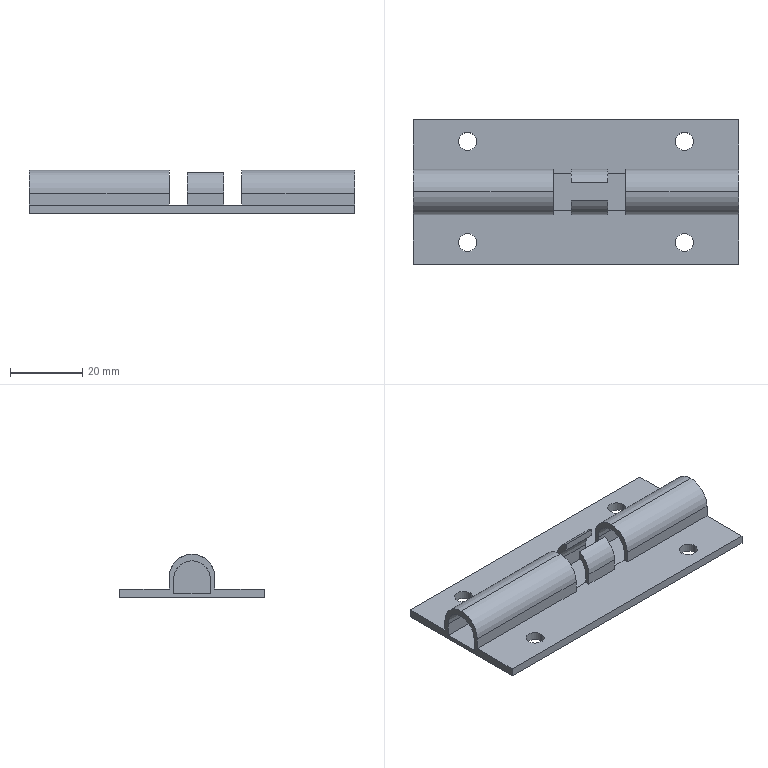Part | SolidWorks | features BaseBody 1 | 1 solid | 45 faces | box 90 x 40 x 12 mm | volume 11713 mm3 | plane 25 | cylinder 20 | commonest cylinder face diameters 5 x8 10.2 x6 12.6 x6
STEP:
#1=CARTESIAN_POINT('',(17.5,14.,2.4));
#2=VERTEX_POINT('',#1);
#3=CARTESIAN_POINT('',(12.5,14.,2.4));
#4=VERTEX_POINT('',#3);
#5=CARTESIAN_POINT('',(15.,14.,2.4));
#6=DIRECTION('',(0.,0.,-1.));
#7=DIRECTION('',(-1.,0.,0.));
#8=AXIS2_PLACEMENT_3D('',#5,#6,#7);
#9=CIRCLE('',#8,2.5);
#10=EDGE_CURVE('',#2,#4,#9,.T.);
#11=ORIENTED_EDGE('',*,*,#10,.F.);
#12=CARTESIAN_POINT('',(17.5,14.,0.));
#13=VERTEX_POINT('',#12);
#14=CARTESIAN_POINT('',(17.5,14.,0.));
#15=DIRECTION('',(0.,0.,-1.));
#16=VECTOR('',#15,1000.);
#17=LINE('',#14,#16);
#18=EDGE_CURVE('',#2,#13,#17,.T.);
#19=ORIENTED_EDGE('',*,*,#18,.T.);
#20=CARTESIAN_POINT('',(12.5,14.,0.));
#21=VERTEX_POINT('',#20);
#22=CARTESIAN_POINT('',(15.,14.,0.));
#23=DIRECTION('',(0.,0.,1.));
#24=DIRECTION('',(-1.,0.,0.));
#25=AXIS2_PLACEMENT_3D('',#22,#23,#24);
#26=CIRCLE('',#25,2.5);
#27=EDGE_CURVE('',#21,#13,#26,.T.);
#28=ORIENTED_EDGE('',*,*,#27,.F.);
#29=CARTESIAN_POINT('',(12.5,14.,0.));
#30=DIRECTION('',(0.,0.,-1.));
#31=VECTOR('',#30,1000.);
#32=LINE('',#29,#31);
#33=EDGE_CURVE('',#4,#21,#32,.T.);
#34=ORIENTED_EDGE('',*,*,#33,.F.);
#35=EDGE_LOOP('',(#11,#19,#28,#34));
#36=FACE_OUTER_BOUND('',#35,.T.);
#37=CARTESIAN_POINT('',(15.,14.,0.));
#38=DIRECTION('',(0.,0.,-1.));
#39=DIRECTION('',(-1.,0.,0.));
#40=AXIS2_PLACEMENT_3D('',#37,#38,#39);
#41=CYLINDRICAL_SURFACE('',#40,2.5);
#42=ADVANCED_FACE('',(#36),#41,.F.);
#43=CARTESIAN_POINT('',(77.5,-14.,2.4));
#44=VERTEX_POINT('',#43);
#45=CARTESIAN_POINT('',(72.5,-14.,2.4));
#46=VERTEX_POINT('',#45);
#47=CARTESIAN_POINT('',(75.,-14.,2.4));
#48=DIRECTION('',(0.,0.,-1.));
#49=DIRECTION('',(-1.,0.,0.));
#50=AXIS2_PLACEMENT_3D('',#47,#48,#49);
#51=CIRCLE('',#50,2.5);
#52=EDGE_CURVE('',#44,#46,#51,.T.);
#53=ORIENTED_EDGE('',*,*,#52,.F.);
#54=CARTESIAN_POINT('',(77.5,-14.,0.));
#55=VERTEX_POINT('',#54);
#56=CARTESIAN_POINT('',(77.5,-14.,0.));
#57=DIRECTION('',(0.,0.,-1.));
#58=VECTOR('',#57,1000.);
#59=LINE('',#56,#58);
#60=EDGE_CURVE('',#44,#55,#59,.T.);
#61=ORIENTED_EDGE('',*,*,#60,.T.);
#62=CARTESIAN_POINT('',(72.5,-14.,0.));
#63=VERTEX_POINT('',#62);
#64=CARTESIAN_POINT('',(75.,-14.,0.));
#65=DIRECTION('',(0.,0.,1.));
#66=DIRECTION('',(-1.,0.,0.));
#67=AXIS2_PLACEMENT_3D('',#64,#65,#66);
#68=CIRCLE('',#67,2.5);
#69=EDGE_CURVE('',#63,#55,#68,.T.);
#70=ORIENTED_EDGE('',*,*,#69,.F.);
#71=CARTESIAN_POINT('',(72.5,-14.,0.));
#72=DIRECTION('',(0.,0.,-1.));
#73=VECTOR('',#72,1000.);
#74=LINE('',#71,#73);
#75=EDGE_CURVE('',#46,#63,#74,.T.);
#76=ORIENTED_EDGE('',*,*,#75,.F.);
#77=EDGE_LOOP('',(#53,#61,#70,#76));
#78=FACE_OUTER_BOUND('',#77,.T.);
#79=CARTESIAN_POINT('',(75.,-14.,0.));
#80=DIRECTION('',(0.,0.,-1.));
#81=DIRECTION('',(-1.,0.,0.));
#82=AXIS2_PLACEMENT_3D('',#79,#80,#81);
#83=CYLINDRICAL_SURFACE('',#82,2.5);
#84=ADVANCED_FACE('',(#78),#83,.F.);
#85=CARTESIAN_POINT('',(17.5,-14.,2.4));
#86=VERTEX_POINT('',#85);
#87=CARTESIAN_POINT('',(12.5,-14.,2.4));
#88=VERTEX_POINT('',#87);
#89=CARTESIAN_POINT('',(15.,-14.,2.4));
#90=DIRECTION('',(0.,0.,-1.));
#91=DIRECTION('',(-1.,0.,0.));
#92=AXIS2_PLACEMENT_3D('',#89,#90,#91);
#93=CIRCLE('',#92,2.5);
#94=EDGE_CURVE('',#86,#88,#93,.T.);
#95=ORIENTED_EDGE('',*,*,#94,.F.);
#96=CARTESIAN_POINT('',(17.5,-14.,0.));
#97=VERTEX_POINT('',#96);
#98=CARTESIAN_POINT('',(17.5,-14.,0.));
#99=DIRECTION('',(0.,0.,-1.));
#100=VECTOR('',#99,1000.);
#101=LINE('',#98,#100);
#102=EDGE_CURVE('',#86,#97,#101,.T.);
#103=ORIENTED_EDGE('',*,*,#102,.T.);
#104=CARTESIAN_POINT('',(12.5,-14.,0.));
#105=VERTEX_POINT('',#104);
#106=CARTESIAN_POINT('',(15.,-14.,0.));
#107=DIRECTION('',(0.,0.,1.));
#108=DIRECTION('',(-1.,0.,0.));
#109=AXIS2_PLACEMENT_3D('',#106,#107,#108);
#110=CIRCLE('',#109,2.5);
#111=EDGE_CURVE('',#105,#97,#110,.T.);
#112=ORIENTED_EDGE('',*,*,#111,.F.);
#113=CARTESIAN_POINT('',(12.5,-14.,0.));
#114=DIRECTION('',(0.,0.,-1.));
#115=VECTOR('',#114,1000.);
#116=LINE('',#113,#115);
#117=EDGE_CURVE('',#88,#105,#116,.T.);
#118=ORIENTED_EDGE('',*,*,#117,.F.);
#119=EDGE_LOOP('',(#95,#103,#112,#118));
#120=FACE_OUTER_BOUND('',#119,.T.);
#121=CARTESIAN_POINT('',(15.,-14.,0.));
#122=DIRECTION('',(0.,0.,-1.));
#123=DIRECTION('',(-1.,0.,0.));
#124=AXIS2_PLACEMENT_3D('',#121,#122,#123);
#125=CYLINDRICAL_SURFACE('',#124,2.5);
#126=ADVANCED_FACE('',(#120),#125,.F.);
#127=CARTESIAN_POINT('',(77.5,14.,2.4));
#128=VERTEX_POINT('',#127);
#129=CARTESIAN_POINT('',(72.5,14.,2.4));
#130=VERTEX_POINT('',#129);
#131=CARTESIAN_POINT('',(75.,14.,2.4));
#132=DIRECTION('',(0.,0.,-1.));
#133=DIRECTION('',(-1.,0.,0.));
#134=AXIS2_PLACEMENT_3D('',#131,#132,#133);
#135=CIRCLE('',#134,2.5);
#136=EDGE_CURVE('',#128,#130,#135,.T.);
#137=ORIENTED_EDGE('',*,*,#136,.F.);
#138=CARTESIAN_POINT('',(77.5,14.,0.));
#139=VERTEX_POINT('',#138);
#140=CARTESIAN_POINT('',(77.5,14.,0.));
#141=DIRECTION('',(0.,0.,-1.));
#142=VECTOR('',#141,1000.);
#143=LINE('',#140,#142);
#144=EDGE_CURVE('',#128,#139,#143,.T.);
#145=ORIENTED_EDGE('',*,*,#144,.T.);
#146=CARTESIAN_POINT('',(72.5,14.,0.));
#147=VERTEX_POINT('',#146);
#148=CARTESIAN_POINT('',(75.,14.,0.));
#149=DIRECTION('',(0.,0.,1.));
#150=DIRECTION('',(-1.,0.,0.));
#151=AXIS2_PLACEMENT_3D('',#148,#149,#150);
#152=CIRCLE('',#151,2.5);
#153=EDGE_CURVE('',#147,#139,#152,.T.);
#154=ORIENTED_EDGE('',*,*,#153,.F.);
#155=CARTESIAN_POINT('',(72.5,14.,0.));
#156=DIRECTION('',(0.,0.,-1.));
#157=VECTOR('',#156,1000.);
#158=LINE('',#155,#157);
#159=EDGE_CURVE('',#130,#147,#158,.T.);
#160=ORIENTED_EDGE('',*,*,#159,.F.);
#161=EDGE_LOOP('',(#137,#145,#154,#160));
#162=FACE_OUTER_BOUND('',#161,.T.);
#163=CARTESIAN_POINT('',(75.,14.,0.));
#164=DIRECTION('',(0.,0.,-1.));
#165=DIRECTION('',(-1.,0.,0.));
#166=AXIS2_PLACEMENT_3D('',#163,#164,#165);
#167=CYLINDRICAL_SURFACE('',#166,2.5);
#168=ADVANCED_FACE('',(#162),#167,.F.);
#169=CARTESIAN_POINT('',(38.75,-6.3,5.7));
#170=VERTEX_POINT('',#169);
#171=CARTESIAN_POINT('',(38.75,0.,12.));
#172=VERTEX_POINT('',#171);
#173=CARTESIAN_POINT('',(38.75,0.,5.7));
#174=DIRECTION('',(-1.,0.,0.));
#175=DIRECTION('',(0.,0.,1.));
#176=AXIS2_PLACEMENT_3D('',#173,#174,#175);
#177=CIRCLE('',#176,6.3);
#178=EDGE_CURVE('',#170,#172,#177,.T.);
#179=ORIENTED_EDGE('',*,*,#178,.T.);
#180=CARTESIAN_POINT('',(0.,0.,12.));
#181=VERTEX_POINT('',#180);
#182=CARTESIAN_POINT('',(0.,0.,12.));
#183=DIRECTION('',(-1.,0.,0.));
#184=VECTOR('',#183,1000.);
#185=LINE('',#182,#184);
#186=EDGE_CURVE('',#172,#181,#185,.T.);
#187=ORIENTED_EDGE('',*,*,#186,.T.);
#188=CARTESIAN_POINT('',(0.,-6.3,5.7));
#189=VERTEX_POINT('',#188);
#190=CARTESIAN_POINT('',(0.,0.,5.7));
#191=DIRECTION('',(1.,0.,0.));
#192=DIRECTION('',(0.,0.,1.));
#193=AXIS2_PLACEMENT_3D('',#190,#191,#192);
#194=CIRCLE('',#193,6.3);
#195=EDGE_CURVE('',#181,#189,#194,.T.);
#196=ORIENTED_EDGE('',*,*,#195,.T.);
#197=CARTESIAN_POINT('',(0.,-6.3,5.7));
#198=DIRECTION('',(1.,0.,0.));
#199=VECTOR('',#198,1000.);
#200=LINE('',#197,#199);
#201=EDGE_CURVE('',#189,#170,#200,.T.);
#202=ORIENTED_EDGE('',*,*,#201,.T.);
#203=EDGE_LOOP('',(#179,#187,#196,#202));
#204=FACE_OUTER_BOUND('',#203,.T.);
#205=CARTESIAN_POINT('',(0.,0.,5.7));
#206=DIRECTION('',(-1.,0.,0.));
#207=DIRECTION('',(0.,0.,1.));
#208=AXIS2_PLACEMENT_3D('',#205,#206,#207);
#209=CYLINDRICAL_SURFACE('',#208,6.3);
#210=ADVANCED_FACE('',(#204),#209,.T.);
#211=CARTESIAN_POINT('',(38.75,0.,10.2));
#212=VERTEX_POINT('',#211);
#213=CARTESIAN_POINT('',(38.75,5.1,5.1));
#214=VERTEX_POINT('',#213);
#215=CARTESIAN_POINT('',(38.75,0.,5.1));
#216=DIRECTION('',(-1.,0.,0.));
#217=DIRECTION('',(0.,0.,1.));
#218=AXIS2_PLACEMENT_3D('',#215,#216,#217);
#219=CIRCLE('',#218,5.1);
#220=EDGE_CURVE('',#212,#214,#219,.T.);
#221=ORIENTED_EDGE('',*,*,#220,.F.);
#222=CARTESIAN_POINT('',(0.,0.,10.2));
#223=VERTEX_POINT('',#222);
#224=CARTESIAN_POINT('',(0.,0.,10.2));
#225=DIRECTION('',(-1.,0.,0.));
#226=VECTOR('',#225,1000.);
#227=LINE('',#224,#226);
#228=EDGE_CURVE('',#212,#223,#227,.T.);
#229=ORIENTED_EDGE('',*,*,#228,.T.);
#230=CARTESIAN_POINT('',(0.,5.1,5.1));
#231=VERTEX_POINT('',#230);
#232=CARTESIAN_POINT('',(0.,0.,5.1));
#233=DIRECTION('',(-1.,0.,0.));
#234=DIRECTION('',(0.,0.,1.));
#235=AXIS2_PLACEMENT_3D('',#232,#233,#234);
#236=CIRCLE('',#235,5.1);
#237=EDGE_CURVE('',#223,#231,#236,.T.);
#238=ORIENTED_EDGE('',*,*,#237,.T.);
#239=CARTESIAN_POINT('',(0.,5.1,5.1));
#240=DIRECTION('',(1.,0.,0.));
#241=VECTOR('',#240,1000.);
#242=LINE('',#239,#241);
#243=EDGE_CURVE('',#231,#214,#242,.T.);
#244=ORIENTED_EDGE('',*,*,#243,.T.);
#245=EDGE_LOOP('',(#221,#229,#238,#244));
#246=FACE_OUTER_BOUND('',#245,.T.);
#247=CARTESIAN_POINT('',(0.,0.,5.1));
#248=DIRECTION('',(-1.,0.,0.));
#249=DIRECTION('',(0.,0.,1.));
#250=AXIS2_PLACEMENT_3D('',#247,#248,#249);
#251=CYLINDRICAL_SURFACE('',#250,5.1);
#252=ADVANCED_FACE('',(#246),#251,.F.);
#253=CARTESIAN_POINT('',(90.,0.,12.));
#254=VERTEX_POINT('',#253);
#255=CARTESIAN_POINT('',(90.,-6.3,5.7));
#256=VERTEX_POINT('',#255);
#257=CARTESIAN_POINT('',(90.,0.,5.7));
#258=DIRECTION('',(1.,0.,0.));
#259=DIRECTION('',(0.,0.,1.));
#260=AXIS2_PLACEMENT_3D('',#257,#258,#259);
#261=CIRCLE('',#260,6.3);
#262=EDGE_CURVE('',#254,#256,#261,.T.);
#263=ORIENTED_EDGE('',*,*,#262,.F.);
#264=CARTESIAN_POINT('',(58.75,0.,12.));
#265=VERTEX_POINT('',#264);
#266=CARTESIAN_POINT('',(0.,0.,12.));
#267=DIRECTION('',(-1.,0.,0.));
#268=VECTOR('',#267,1000.);
#269=LINE('',#266,#268);
#270=EDGE_CURVE('',#254,#265,#269,.T.);
#271=ORIENTED_EDGE('',*,*,#270,.T.);
#272=CARTESIAN_POINT('',(58.75,-6.3,5.7));
#273=VERTEX_POINT('',#272);
#274=CARTESIAN_POINT('',(58.75,0.,5.7));
#275=DIRECTION('',(1.,0.,0.));
#276=DIRECTION('',(0.,0.,1.));
#277=AXIS2_PLACEMENT_3D('',#274,#275,#276);
#278=CIRCLE('',#277,6.3);
#279=EDGE_CURVE('',#265,#273,#278,.T.);
#280=ORIENTED_EDGE('',*,*,#279,.T.);
#281=CARTESIAN_POINT('',(0.,-6.3,5.7));
#282=DIRECTION('',(-1.,0.,0.));
#283=VECTOR('',#282,1000.);
#284=LINE('',#281,#283);
#285=EDGE_CURVE('',#256,#273,#284,.T.);
#286=ORIENTED_EDGE('',*,*,#285,.F.);
#287=EDGE_LOOP('',(#263,#271,#280,#286));
#288=FACE_OUTER_BOUND('',#287,.T.);
#289=CARTESIAN_POINT('',(0.,0.,5.7));
#290=DIRECTION('',(-1.,0.,0.));
#291=DIRECTION('',(0.,0.,1.));
#292=AXIS2_PLACEMENT_3D('',#289,#290,#291);
#293=CYLINDRICAL_SURFACE('',#292,6.3);
#294=ADVANCED_FACE('',(#288),#293,.T.);
#295=CARTESIAN_POINT('',(70.,5.1,5.1));
#296=VERTEX_POINT('',#295);
#297=CARTESIAN_POINT('',(70.,0.,10.2));
#298=VERTEX_POINT('',#297);
#299=CARTESIAN_POINT('',(70.,0.,5.1));
#300=DIRECTION('',(1.,0.,0.));
#301=DIRECTION('',(0.,0.,1.));
#302=AXIS2_PLACEMENT_3D('',#299,#300,#301);
#303=CIRCLE('',#302,5.1);
#304=EDGE_CURVE('',#296,#298,#303,.T.);
#305=ORIENTED_EDGE('',*,*,#304,.T.);
#306=CARTESIAN_POINT('',(58.75,0.,10.2));
#307=VERTEX_POINT('',#306);
#308=CARTESIAN_POINT('',(0.,0.,10.2));
#309=DIRECTION('',(-1.,0.,0.));
#310=VECTOR('',#309,1000.);
#311=LINE('',#308,#310);
#312=EDGE_CURVE('',#298,#307,#311,.T.);
#313=ORIENTED_EDGE('',*,*,#312,.T.);
#314=CARTESIAN_POINT('',(58.75,5.1,5.1));
#315=VERTEX_POINT('',#314);
#316=CARTESIAN_POINT('',(58.75,0.,5.1));
#317=DIRECTION('',(1.,0.,0.));
#318=DIRECTION('',(0.,0.,1.));
#319=AXIS2_PLACEMENT_3D('',#316,#317,#318);
#320=CIRCLE('',#319,5.1);
#321=EDGE_CURVE('',#315,#307,#320,.T.);
#322=ORIENTED_EDGE('',*,*,#321,.F.);
#323=CARTESIAN_POINT('',(0.,5.1,5.1));
#324=DIRECTION('',(1.,0.,0.));
#325=VECTOR('',#324,1000.);
#326=LINE('',#323,#325);
#327=EDGE_CURVE('',#315,#296,#326,.T.);
#328=ORIENTED_EDGE('',*,*,#327,.T.);
#329=EDGE_LOOP('',(#305,#313,#322,#328));
#330=FACE_OUTER_BOUND('',#329,.T.);
#331=CARTESIAN_POINT('',(0.,0.,5.1));
#332=DIRECTION('',(-1.,0.,0.));
#333=DIRECTION('',(0.,0.,1.));
#334=AXIS2_PLACEMENT_3D('',#331,#332,#333);
#335=CYLINDRICAL_SURFACE('',#334,5.1);
#336=ADVANCED_FACE('',(#330),#335,.F.);
#337=CARTESIAN_POINT('',(43.75,-2.5,9.545));
#338=VERTEX_POINT('',#337);
#339=CARTESIAN_POINT('',(43.75,-2.5,11.483));
#340=VERTEX_POINT('',#339);
#341=CARTESIAN_POINT('',(43.75,-2.5,2.4));
#342=DIRECTION('',(0.,0.,1.));
#343=VECTOR('',#342,1000.);
#344=LINE('',#341,#343);
#345=EDGE_CURVE('',#338,#340,#344,.T.);
#346=ORIENTED_EDGE('',*,*,#345,.T.);
#347=CARTESIAN_POINT('',(53.75,-2.5,11.483));
#348=VERTEX_POINT('',#347);
#349=CARTESIAN_POINT('',(0.,-2.5,11.483));
#350=DIRECTION('',(-1.,0.,0.));
#351=VECTOR('',#350,1000.);
#352=LINE('',#349,#351);
#353=EDGE_CURVE('',#348,#340,#352,.T.);
#354=ORIENTED_EDGE('',*,*,#353,.F.);
#355=CARTESIAN_POINT('',(53.75,-2.5,9.545));
#356=VERTEX_POINT('',#355);
#357=CARTESIAN_POINT('',(53.75,-2.5,2.4));
#358=DIRECTION('',(0.,0.,-1.));
#359=VECTOR('',#358,1000.);
#360=LINE('',#357,#359);
#361=EDGE_CURVE('',#348,#356,#360,.T.);
#362=ORIENTED_EDGE('',*,*,#361,.T.);
#363=CARTESIAN_POINT('',(0.,-2.5,9.545));
#364=DIRECTION('',(-1.,0.,0.));
#365=VECTOR('',#364,1000.);
#366=LINE('',#363,#365);
#367=EDGE_CURVE('',#356,#338,#366,.T.);
#368=ORIENTED_EDGE('',*,*,#367,.T.);
#369=EDGE_LOOP('',(#346,#354,#362,#368));
#370=FACE_OUTER_BOUND('',#369,.T.);
#371=CARTESIAN_POINT('',(53.75,-2.5,2.4));
#372=DIRECTION('',(0.,-1.,0.));
#373=DIRECTION('',(0.,0.,-1.));
#374=AXIS2_PLACEMENT_3D('',#371,#372,#373);
#375=PLANE('',#374);
#376=ADVANCED_FACE('',(#370),#375,.F.);
#377=CARTESIAN_POINT('',(53.75,2.5,9.545));
#378=VERTEX_POINT('',#377);
#379=CARTESIAN_POINT('',(53.75,2.5,11.483));
#380=VERTEX_POINT('',#379);
#381=CARTESIAN_POINT('',(53.75,2.5,2.4));
#382=DIRECTION('',(0.,0.,1.));
#383=VECTOR('',#382,1000.);
#384=LINE('',#381,#383);
#385=EDGE_CURVE('',#378,#380,#384,.T.);
#386=ORIENTED_EDGE('',*,*,#385,.T.);
#387=CARTESIAN_POINT('',(43.75,2.5,11.483));
#388=VERTEX_POINT('',#387);
#389=CARTESIAN_POINT('',(0.,2.5,11.483));
#390=DIRECTION('',(1.,0.,0.));
#391=VECTOR('',#390,1000.);
#392=LINE('',#389,#391);
#393=EDGE_CURVE('',#388,#380,#392,.T.);
#394=ORIENTED_EDGE('',*,*,#393,.F.);
#395=CARTESIAN_POINT('',(43.75,2.5,9.545));
#396=VERTEX_POINT('',#395);
#397=CARTESIAN_POINT('',(43.75,2.5,2.4));
#398=DIRECTION('',(0.,0.,-1.));
#399=VECTOR('',#398,1000.);
#400=LINE('',#397,#399);
#401=EDGE_CURVE('',#388,#396,#400,.T.);
#402=ORIENTED_EDGE('',*,*,#401,.T.);
#403=CARTESIAN_POINT('',(0.,2.5,9.545));
#404=DIRECTION('',(1.,0.,0.));
#405=VECTOR('',#404,1000.);
#406=LINE('',#403,#405);
#407=EDGE_CURVE('',#396,#378,#406,.T.);
#408=ORIENTED_EDGE('',*,*,#407,.T.);
#409=EDGE_LOOP('',(#386,#394,#402,#408));
#410=FACE_OUTER_BOUND('',#409,.T.);
#411=CARTESIAN_POINT('',(43.75,2.5,2.4));
#412=DIRECTION('',(0.,1.,0.));
#413=DIRECTION('',(1.,0.,0.));
#414=AXIS2_PLACEMENT_3D('',#411,#412,#413);
#415=PLANE('',#414);
#416=ADVANCED_FACE('',(#410),#415,.F.);
#417=CARTESIAN_POINT('',(43.75,-6.3,5.7));
#418=VERTEX_POINT('',#417);
#419=CARTESIAN_POINT('',(43.75,0.,5.7));
#420=DIRECTION('',(1.,0.,0.));
#421=DIRECTION('',(0.,0.,1.));
#422=AXIS2_PLACEMENT_3D('',#419,#420,#421);
#423=CIRCLE('',#422,6.3);
#424=EDGE_CURVE('',#340,#418,#423,.T.);
#425=ORIENTED_EDGE('',*,*,#424,.T.);
#426=CARTESIAN_POINT('',(53.75,-6.3,5.7));
#427=VERTEX_POINT('',#426);
#428=CARTESIAN_POINT('',(0.,-6.3,5.7));
#429=DIRECTION('',(-1.,0.,0.));
#430=VECTOR('',#429,1000.);
#431=LINE('',#428,#430);
#432=EDGE_CURVE('',#427,#418,#431,.T.);
#433=ORIENTED_EDGE('',*,*,#432,.F.);
#434=CARTESIAN_POINT('',(53.75,0.,5.7));
#435=DIRECTION('',(-1.,0.,0.));
#436=DIRECTION('',(0.,0.,1.));
#437=AXIS2_PLACEMENT_3D('',#434,#435,#436);
#438=CIRCLE('',#437,6.3);
#439=EDGE_CURVE('',#427,#348,#438,.T.);
#440=ORIENTED_EDGE('',*,*,#439,.T.);
#441=ORIENTED_EDGE('',*,*,#353,.T.);
#442=EDGE_LOOP('',(#425,#433,#440,#441));
#443=FACE_OUTER_BOUND('',#442,.T.);
#444=CARTESIAN_POINT('',(0.,0.,5.7));
#445=DIRECTION('',(-1.,0.,0.));
#446=DIRECTION('',(0.,0.,1.));
#447=AXIS2_PLACEMENT_3D('',#444,#445,#446);
#448=CYLINDRICAL_SURFACE('',#447,6.3);
#449=ADVANCED_FACE('',(#443),#448,.T.);
#450=CARTESIAN_POINT('',(43.75,6.3,5.7));
#451=VERTEX_POINT('',#450);
#452=CARTESIAN_POINT('',(43.75,0.,5.7));
#453=DIRECTION('',(1.,0.,0.));
#454=DIRECTION('',(0.,0.,1.));
#455=AXIS2_PLACEMENT_3D('',#452,#453,#454);
#456=CIRCLE('',#455,6.3);
#457=EDGE_CURVE('',#451,#388,#456,.T.);
#458=ORIENTED_EDGE('',*,*,#457,.T.);
#459=ORIENTED_EDGE('',*,*,#393,.T.);
#460=CARTESIAN_POINT('',(53.75,6.3,5.7));
#461=VERTEX_POINT('',#460);
#462=CARTESIAN_POINT('',(53.75,0.,5.7));
#463=DIRECTION('',(-1.,0.,0.));
#464=DIRECTION('',(0.,0.,1.));
#465=AXIS2_PLACEMENT_3D('',#462,#463,#464);
#466=CIRCLE('',#465,6.3);
#467=EDGE_CURVE('',#380,#461,#466,.T.);
#468=ORIENTED_EDGE('',*,*,#467,.T.);
#469=CARTESIAN_POINT('',(0.,6.3,5.7));
#470=DIRECTION('',(1.,0.,0.));
#471=VECTOR('',#470,1000.);
#472=LINE('',#469,#471);
#473=EDGE_CURVE('',#451,#461,#472,.T.);
#474=ORIENTED_EDGE('',*,*,#473,.F.);
#475=EDGE_LOOP('',(#458,#459,#468,#474));
#476=FACE_OUTER_BOUND('',#475,.T.);
#477=CARTESIAN_POINT('',(0.,0.,5.7));
#478=DIRECTION('',(-1.,0.,0.));
#479=DIRECTION('',(0.,0.,1.));
#480=AXIS2_PLACEMENT_3D('',#477,#478,#479);
#481=CYLINDRICAL_SURFACE('',#480,6.3);
#482=ADVANCED_FACE('',(#476),#481,.T.);
#483=CARTESIAN_POINT('',(53.75,-5.1,5.1));
#484=VERTEX_POINT('',#483);
#485=CARTESIAN_POINT('',(53.75,0.,5.1));
#486=DIRECTION('',(-1.,0.,0.));
#487=DIRECTION('',(0.,0.,1.));
#488=AXIS2_PLACEMENT_3D('',#485,#486,#487);
#489=CIRCLE('',#488,5.1);
#490=EDGE_CURVE('',#484,#356,#489,.T.);
#491=ORIENTED_EDGE('',*,*,#490,.T.);
#492=ORIENTED_EDGE('',*,*,#361,.F.);
#493=ORIENTED_EDGE('',*,*,#439,.F.);
#494=CARTESIAN_POINT('',(53.75,-6.3,2.4));
#495=VERTEX_POINT('',#494);
#496=CARTESIAN_POINT('',(53.75,-6.3,2.4));
#497=DIRECTION('',(0.,0.,1.));
#498=VECTOR('',#497,1000.);
#499=LINE('',#496,#498);
#500=EDGE_CURVE('',#495,#427,#499,.T.);
#501=ORIENTED_EDGE('',*,*,#500,.F.);
#502=CARTESIAN_POINT('',(53.75,-5.1,2.4));
#503=VERTEX_POINT('',#502);
#504=CARTESIAN_POINT('',(53.75,-6.3,2.4));
#505=DIRECTION('',(0.,-1.,0.));
#506=VECTOR('',#505,1000.);
#507=LINE('',#504,#506);
#508=EDGE_CURVE('',#503,#495,#507,.T.);
#509=ORIENTED_EDGE('',*,*,#508,.F.);
#510=CARTESIAN_POINT('',(53.75,-5.1,1.2));
#511=DIRECTION('',(0.,0.,1.));
#512=VECTOR('',#511,1000.);
#513=LINE('',#510,#512);
#514=EDGE_CURVE('',#503,#484,#513,.T.);
#515=ORIENTED_EDGE('',*,*,#514,.T.);
#516=EDGE_LOOP('',(#491,#492,#493,#501,#509,#515));
#517=FACE_OUTER_BOUND('',#516,.T.);
#518=CARTESIAN_POINT('',(53.75,-6.3,2.4));
#519=DIRECTION('',(-1.,0.,0.));
#520=DIRECTION('',(0.,0.,1.));
#521=AXIS2_PLACEMENT_3D('',#518,#519,#520);
#522=PLANE('',#521);
#523=ADVANCED_FACE('',(#517),#522,.F.);
#524=CARTESIAN_POINT('',(43.75,-5.1,5.1));
#525=VERTEX_POINT('',#524);
#526=CARTESIAN_POINT('',(0.,-5.1,5.1));
#527=DIRECTION('',(-1.,0.,0.));
#528=VECTOR('',#527,1000.);
#529=LINE('',#526,#528);
#530=EDGE_CURVE('',#484,#525,#529,.T.);
#531=ORIENTED_EDGE('',*,*,#530,.T.);
#532=CARTESIAN_POINT('',(43.75,0.,5.1));
#533=DIRECTION('',(-1.,0.,0.));
#534=DIRECTION('',(0.,0.,1.));
#535=AXIS2_PLACEMENT_3D('',#532,#533,#534);
#536=CIRCLE('',#535,5.1);
#537=EDGE_CURVE('',#525,#338,#536,.T.);
#538=ORIENTED_EDGE('',*,*,#537,.T.);
#539=ORIENTED_EDGE('',*,*,#367,.F.);
#540=ORIENTED_EDGE('',*,*,#490,.F.);
#541=EDGE_LOOP('',(#531,#538,#539,#540));
#542=FACE_OUTER_BOUND('',#541,.T.);
#543=CARTESIAN_POINT('',(0.,0.,5.1));
#544=DIRECTION('',(-1.,0.,0.));
#545=DIRECTION('',(0.,0.,1.));
#546=AXIS2_PLACEMENT_3D('',#543,#544,#545);
#547=CYLINDRICAL_SURFACE('',#546,5.1);
#548=ADVANCED_FACE('',(#542),#547,.F.);
#549=CARTESIAN_POINT('',(43.75,-5.1,2.4));
#550=VERTEX_POINT('',#549);
#551=CARTESIAN_POINT('',(43.75,-5.1,1.2));
#552=DIRECTION('',(0.,0.,-1.));
#553=VECTOR('',#552,1000.);
#554=LINE('',#551,#553);
#555=EDGE_CURVE('',#525,#550,#554,.T.);
#556=ORIENTED_EDGE('',*,*,#555,.T.);
#557=CARTESIAN_POINT('',(43.75,-6.3,2.4));
#558=VERTEX_POINT('',#557);
#559=CARTESIAN_POINT('',(43.75,-2.5,2.4));
#560=DIRECTION('',(0.,1.,0.));
#561=VECTOR('',#560,1000.);
#562=LINE('',#559,#561);
#563=EDGE_CURVE('',#558,#550,#562,.T.);
#564=ORIENTED_EDGE('',*,*,#563,.F.);
#565=CARTESIAN_POINT('',(43.75,-6.3,2.4));
#566=DIRECTION('',(0.,0.,-1.));
#567=VECTOR('',#566,1000.);
#568=LINE('',#565,#567);
#569=EDGE_CURVE('',#418,#558,#568,.T.);
#570=ORIENTED_EDGE('',*,*,#569,.F.);
#571=ORIENTED_EDGE('',*,*,#424,.F.);
#572=ORIENTED_EDGE('',*,*,#345,.F.);
#573=ORIENTED_EDGE('',*,*,#537,.F.);
#574=EDGE_LOOP('',(#556,#564,#570,#571,#572,#573));
#575=FACE_OUTER_BOUND('',#574,.T.);
#576=CARTESIAN_POINT('',(43.75,-2.5,2.4));
#577=DIRECTION('',(1.,0.,0.));
#578=DIRECTION('',(0.,1.,0.));
#579=AXIS2_PLACEMENT_3D('',#576,#577,#578);
#580=PLANE('',#579);
#581=ADVANCED_FACE('',(#575),#580,.F.);
#582=ORIENTED_EDGE('',*,*,#321,.T.);
#583=CARTESIAN_POINT('',(58.75,-5.1,5.1));
#584=VERTEX_POINT('',#583);
#585=CARTESIAN_POINT('',(58.75,0.,5.1));
#586=DIRECTION('',(1.,0.,0.));
#587=DIRECTION('',(0.,0.,1.));
#588=AXIS2_PLACEMENT_3D('',#585,#586,#587);
#589=CIRCLE('',#588,5.1);
#590=EDGE_CURVE('',#307,#584,#589,.T.);
#591=ORIENTED_EDGE('',*,*,#590,.T.);
#592=CARTESIAN_POINT('',(58.75,-5.1,2.4));
#593=VERTEX_POINT('',#592);
#594=CARTESIAN_POINT('',(58.75,-5.1,1.2));
#595=DIRECTION('',(0.,0.,-1.));
#596=VECTOR('',#595,1000.);
#597=LINE('',#594,#596);
#598=EDGE_CURVE('',#584,#593,#597,.T.);
#599=ORIENTED_EDGE('',*,*,#598,.T.);
#600=CARTESIAN_POINT('',(58.75,-6.3,2.4));
#601=VERTEX_POINT('',#600);
#602=CARTESIAN_POINT('',(58.75,6.3,2.4));
#603=DIRECTION('',(0.,1.,0.));
#604=VECTOR('',#603,1000.);
#605=LINE('',#602,#604);
#606=EDGE_CURVE('',#601,#593,#605,.T.);
#607=ORIENTED_EDGE('',*,*,#606,.F.);
#608=CARTESIAN_POINT('',(58.75,-6.3,2.4));
#609=DIRECTION('',(0.,0.,-1.));
#610=VECTOR('',#609,1000.);
#611=LINE('',#608,#610);
#612=EDGE_CURVE('',#273,#601,#611,.T.);
#613=ORIENTED_EDGE('',*,*,#612,.F.);
#614=ORIENTED_EDGE('',*,*,#279,.F.);
#615=CARTESIAN_POINT('',(58.75,6.3,5.7));
#616=VERTEX_POINT('',#615);
#617=CARTESIAN_POINT('',(58.75,0.,5.7));
#618=DIRECTION('',(1.,0.,0.));
#619=DIRECTION('',(0.,0.,1.));
#620=AXIS2_PLACEMENT_3D('',#617,#618,#619);
#621=CIRCLE('',#620,6.3);
#622=EDGE_CURVE('',#616,#265,#621,.T.);
#623=ORIENTED_EDGE('',*,*,#622,.F.);
#624=CARTESIAN_POINT('',(58.75,6.3,2.4));
#625=VERTEX_POINT('',#624);
#626=CARTESIAN_POINT('',(58.75,6.3,5.7));
#627=DIRECTION('',(0.,0.,1.));
#628=VECTOR('',#627,1000.);
#629=LINE('',#626,#628);
#630=EDGE_CURVE('',#625,#616,#629,.T.);
#631=ORIENTED_EDGE('',*,*,#630,.F.);
#632=CARTESIAN_POINT('',(58.75,5.1,2.4));
#633=VERTEX_POINT('',#632);
#634=CARTESIAN_POINT('',(58.75,6.3,2.4));
#635=DIRECTION('',(0.,1.,0.));
#636=VECTOR('',#635,1000.);
#637=LINE('',#634,#636);
#638=EDGE_CURVE('',#633,#625,#637,.T.);
#639=ORIENTED_EDGE('',*,*,#638,.F.);
#640=CARTESIAN_POINT('',(58.75,5.1,5.1));
#641=DIRECTION('',(0.,0.,1.));
#642=VECTOR('',#641,1000.);
#643=LINE('',#640,#642);
#644=EDGE_CURVE('',#633,#315,#643,.T.);
#645=ORIENTED_EDGE('',*,*,#644,.T.);
#646=EDGE_LOOP('',(#582,#591,#599,#607,#613,#614,#623,#631,#639,#645));
#647=FACE_OUTER_BOUND('',#646,.T.);
#648=CARTESIAN_POINT('',(58.75,6.3,2.4));
#649=DIRECTION('',(1.,0.,0.));
#650=DIRECTION('',(0.,1.,0.));
#651=AXIS2_PLACEMENT_3D('',#648,#649,#650);
#652=PLANE('',#651);
#653=ADVANCED_FACE('',(#647),#652,.F.);
#654=CARTESIAN_POINT('',(70.,5.1,1.2));
#655=VERTEX_POINT('',#654);
#656=CARTESIAN_POINT('',(70.,-5.1,1.2));
#657=VERTEX_POINT('',#656);
#658=CARTESIAN_POINT('',(70.,5.1,1.2));
#659=DIRECTION('',(0.,-1.,0.));
#660=VECTOR('',#659,1000.);
#661=LINE('',#658,#660);
#662=EDGE_CURVE('',#655,#657,#661,.T.);
#663=ORIENTED_EDGE('',*,*,#662,.T.);
#664=CARTESIAN_POINT('',(70.,-5.1,5.1));
#665=VERTEX_POINT('',#664);
#666=CARTESIAN_POINT('',(70.,-5.1,1.2));
#667=DIRECTION('',(0.,0.,1.));
#668=VECTOR('',#667,1000.);
#669=LINE('',#666,#668);
#670=EDGE_CURVE('',#657,#665,#669,.T.);
#671=ORIENTED_EDGE('',*,*,#670,.T.);
#672=CARTESIAN_POINT('',(70.,0.,5.1));
#673=DIRECTION('',(1.,0.,0.));
#674=DIRECTION('',(0.,0.,1.));
#675=AXIS2_PLACEMENT_3D('',#672,#673,#674);
#676=CIRCLE('',#675,5.1);
#677=EDGE_CURVE('',#298,#665,#676,.T.);
#678=ORIENTED_EDGE('',*,*,#677,.F.);
#679=ORIENTED_EDGE('',*,*,#304,.F.);
#680=CARTESIAN_POINT('',(70.,5.1,5.1));
#681=DIRECTION('',(0.,0.,-1.));
#682=VECTOR('',#681,1000.);
#683=LINE('',#680,#682);
#684=EDGE_CURVE('',#296,#655,#683,.T.);
#685=ORIENTED_EDGE('',*,*,#684,.T.);
#686=EDGE_LOOP('',(#663,#671,#678,#679,#685));
#687=FACE_OUTER_BOUND('',#686,.T.);
#688=CARTESIAN_POINT('',(70.,0.,0.));
#689=DIRECTION('',(1.,0.,0.));
#690=DIRECTION('',(0.,1.,0.));
#691=AXIS2_PLACEMENT_3D('',#688,#689,#690);
#692=PLANE('',#691);
#693=ADVANCED_FACE('',(#687),#692,.F.);
#694=ORIENTED_EDGE('',*,*,#401,.F.);
#695=ORIENTED_EDGE('',*,*,#457,.F.);
#696=CARTESIAN_POINT('',(43.75,6.3,2.4));
#697=VERTEX_POINT('',#696);
#698=CARTESIAN_POINT('',(43.75,6.3,5.7));
#699=DIRECTION('',(0.,0.,1.));
#700=VECTOR('',#699,1000.);
#701=LINE('',#698,#700);
#702=EDGE_CURVE('',#697,#451,#701,.T.);
#703=ORIENTED_EDGE('',*,*,#702,.F.);
#704=CARTESIAN_POINT('',(43.75,5.1,2.4));
#705=VERTEX_POINT('',#704);
#706=CARTESIAN_POINT('',(43.75,6.3,2.4));
#707=DIRECTION('',(0.,1.,0.));
#708=VECTOR('',#707,1000.);
#709=LINE('',#706,#708);
#710=EDGE_CURVE('',#705,#697,#709,.T.);
#711=ORIENTED_EDGE('',*,*,#710,.F.);
#712=CARTESIAN_POINT('',(43.75,5.1,5.1));
#713=VERTEX_POINT('',#712);
#714=CARTESIAN_POINT('',(43.75,5.1,5.1));
#715=DIRECTION('',(0.,0.,1.));
#716=VECTOR('',#715,1000.);
#717=LINE('',#714,#716);
#718=EDGE_CURVE('',#705,#713,#717,.T.);
#719=ORIENTED_EDGE('',*,*,#718,.T.);
#720=CARTESIAN_POINT('',(43.75,0.,5.1));
#721=DIRECTION('',(1.,0.,0.));
#722=DIRECTION('',(0.,0.,1.));
#723=AXIS2_PLACEMENT_3D('',#720,#721,#722);
#724=CIRCLE('',#723,5.1);
#725=EDGE_CURVE('',#713,#396,#724,.T.);
#726=ORIENTED_EDGE('',*,*,#725,.T.);
#727=EDGE_LOOP('',(#694,#695,#703,#711,#719,#726));
#728=FACE_OUTER_BOUND('',#727,.T.);
#729=CARTESIAN_POINT('',(43.75,6.3,2.4));
#730=DIRECTION('',(1.,0.,0.));
#731=DIRECTION('',(0.,1.,0.));
#732=AXIS2_PLACEMENT_3D('',#729,#730,#731);
#733=PLANE('',#732);
#734=ADVANCED_FACE('',(#728),#733,.F.);
#735=ORIENTED_EDGE('',*,*,#407,.F.);
#736=ORIENTED_EDGE('',*,*,#725,.F.);
#737=CARTESIAN_POINT('',(53.75,5.1,5.1));
#738=VERTEX_POINT('',#737);
#739=CARTESIAN_POINT('',(0.,5.1,5.1));
#740=DIRECTION('',(1.,0.,0.));
#741=VECTOR('',#740,1000.);
#742=LINE('',#739,#741);
#743=EDGE_CURVE('',#713,#738,#742,.T.);
#744=ORIENTED_EDGE('',*,*,#743,.T.);
#745=CARTESIAN_POINT('',(53.75,0.,5.1));
#746=DIRECTION('',(1.,0.,0.));
#747=DIRECTION('',(0.,0.,1.));
#748=AXIS2_PLACEMENT_3D('',#745,#746,#747);
#749=CIRCLE('',#748,5.1);
#750=EDGE_CURVE('',#738,#378,#749,.T.);
#751=ORIENTED_EDGE('',*,*,#750,.T.);
#752=EDGE_LOOP('',(#735,#736,#744,#751));
#753=FACE_OUTER_BOUND('',#752,.T.);
#754=CARTESIAN_POINT('',(0.,0.,5.1));
#755=DIRECTION('',(-1.,0.,0.));
#756=DIRECTION('',(0.,0.,1.));
#757=AXIS2_PLACEMENT_3D('',#754,#755,#756);
#758=CYLINDRICAL_SURFACE('',#757,5.1);
#759=ADVANCED_FACE('',(#753),#758,.F.);
#760=CARTESIAN_POINT('',(53.75,6.3,2.4));
#761=VERTEX_POINT('',#760);
#762=CARTESIAN_POINT('',(53.75,5.1,2.4));
#763=VERTEX_POINT('',#762);
#764=CARTESIAN_POINT('',(53.75,2.5,2.4));
#765=DIRECTION('',(0.,-1.,0.));
#766=VECTOR('',#765,1000.);
#767=LINE('',#764,#766);
#768=EDGE_CURVE('',#761,#763,#767,.T.);
#769=ORIENTED_EDGE('',*,*,#768,.F.);
#770=CARTESIAN_POINT('',(53.75,6.3,5.7));
#771=DIRECTION('',(0.,0.,-1.));
#772=VECTOR('',#771,1000.);
#773=LINE('',#770,#772);
#774=EDGE_CURVE('',#461,#761,#773,.T.);
#775=ORIENTED_EDGE('',*,*,#774,.F.);
#776=ORIENTED_EDGE('',*,*,#467,.F.);
#777=ORIENTED_EDGE('',*,*,#385,.F.);
#778=ORIENTED_EDGE('',*,*,#750,.F.);
#779=CARTESIAN_POINT('',(53.75,5.1,5.1));
#780=DIRECTION('',(0.,0.,-1.));
#781=VECTOR('',#780,1000.);
#782=LINE('',#779,#781);
#783=EDGE_CURVE('',#738,#763,#782,.T.);
#784=ORIENTED_EDGE('',*,*,#783,.T.);
#785=EDGE_LOOP('',(#769,#775,#776,#777,#778,#784));
#786=FACE_OUTER_BOUND('',#785,.T.);
#787=CARTESIAN_POINT('',(53.75,2.5,2.4));
#788=DIRECTION('',(-1.,0.,0.));
#789=DIRECTION('',(0.,0.,1.));
#790=AXIS2_PLACEMENT_3D('',#787,#788,#789);
#791=PLANE('',#790);
#792=ADVANCED_FACE('',(#786),#791,.F.);
#793=ORIENTED_EDGE('',*,*,#569,.T.);
#794=CARTESIAN_POINT('',(0.,-6.3,2.4));
#795=DIRECTION('',(-1.,0.,0.));
#796=VECTOR('',#795,1000.);
#797=LINE('',#794,#796);
#798=EDGE_CURVE('',#495,#558,#797,.T.);
#799=ORIENTED_EDGE('',*,*,#798,.F.);
#800=ORIENTED_EDGE('',*,*,#500,.T.);
#801=ORIENTED_EDGE('',*,*,#432,.T.);
#802=EDGE_LOOP('',(#793,#799,#800,#801));
#803=FACE_OUTER_BOUND('',#802,.T.);
#804=CARTESIAN_POINT('',(0.,-6.3,2.4));
#805=DIRECTION('',(0.,-1.,0.));
#806=DIRECTION('',(0.,0.,-1.));
#807=AXIS2_PLACEMENT_3D('',#804,#805,#806);
#808=PLANE('',#807);
#809=ADVANCED_FACE('',(#803),#808,.T.);
#810=CARTESIAN_POINT('',(38.75,6.3,2.4));
#811=VERTEX_POINT('',#810);
#812=CARTESIAN_POINT('',(38.75,5.1,2.4));
#813=VERTEX_POINT('',#812);
#814=CARTESIAN_POINT('',(38.75,-6.3,2.4));
#815=DIRECTION('',(0.,-1.,0.));
#816=VECTOR('',#815,1000.);
#817=LINE('',#814,#816);
#818=EDGE_CURVE('',#811,#813,#817,.T.);
#819=ORIENTED_EDGE('',*,*,#818,.F.);
#820=CARTESIAN_POINT('',(38.75,6.3,5.7));
#821=VERTEX_POINT('',#820);
#822=CARTESIAN_POINT('',(38.75,6.3,5.7));
#823=DIRECTION('',(0.,0.,-1.));
#824=VECTOR('',#823,1000.);
#825=LINE('',#822,#824);
#826=EDGE_CURVE('',#821,#811,#825,.T.);
#827=ORIENTED_EDGE('',*,*,#826,.F.);
#828=CARTESIAN_POINT('',(38.75,0.,5.7));
#829=DIRECTION('',(-1.,0.,0.));
#830=DIRECTION('',(0.,0.,1.));
#831=AXIS2_PLACEMENT_3D('',#828,#829,#830);
#832=CIRCLE('',#831,6.3);
#833=EDGE_CURVE('',#172,#821,#832,.T.);
#834=ORIENTED_EDGE('',*,*,#833,.F.);
#835=ORIENTED_EDGE('',*,*,#178,.F.);
#836=CARTESIAN_POINT('',(38.75,-6.3,2.4));
#837=VERTEX_POINT('',#836);
#838=CARTESIAN_POINT('',(38.75,-6.3,2.4));
#839=DIRECTION('',(0.,0.,1.));
#840=VECTOR('',#839,1000.);
#841=LINE('',#838,#840);
#842=EDGE_CURVE('',#837,#170,#841,.T.);
#843=ORIENTED_EDGE('',*,*,#842,.F.);
#844=CARTESIAN_POINT('',(38.75,-5.1,2.4));
#845=VERTEX_POINT('',#844);
#846=CARTESIAN_POINT('',(38.75,-20.,2.4));
#847=DIRECTION('',(0.,-1.,0.));
#848=VECTOR('',#847,1000.);
#849=LINE('',#846,#848);
#850=EDGE_CURVE('',#845,#837,#849,.T.);
#851=ORIENTED_EDGE('',*,*,#850,.F.);
#852=CARTESIAN_POINT('',(38.75,-5.1,5.1));
#853=VERTEX_POINT('',#852);
#854=CARTESIAN_POINT('',(38.75,-5.1,1.2));
#855=DIRECTION('',(0.,0.,1.));
#856=VECTOR('',#855,1000.);
#857=LINE('',#854,#856);
#858=EDGE_CURVE('',#845,#853,#857,.T.);
#859=ORIENTED_EDGE('',*,*,#858,.T.);
#860=CARTESIAN_POINT('',(38.75,0.,5.1));
#861=DIRECTION('',(-1.,0.,0.));
#862=DIRECTION('',(0.,0.,1.));
#863=AXIS2_PLACEMENT_3D('',#860,#861,#862);
#864=CIRCLE('',#863,5.1);
#865=EDGE_CURVE('',#853,#212,#864,.T.);
#866=ORIENTED_EDGE('',*,*,#865,.T.);
#867=ORIENTED_EDGE('',*,*,#220,.T.);
#868=CARTESIAN_POINT('',(38.75,5.1,5.1));
#869=DIRECTION('',(0.,0.,-1.));
#870=VECTOR('',#869,1000.);
#871=LINE('',#868,#870);
#872=EDGE_CURVE('',#214,#813,#871,.T.);
#873=ORIENTED_EDGE('',*,*,#872,.T.);
#874=EDGE_LOOP('',(#819,#827,#834,#835,#843,#851,#859,#866,#867,#873));
#875=FACE_OUTER_BOUND('',#874,.T.);
#876=CARTESIAN_POINT('',(38.75,-6.3,2.4));
#877=DIRECTION('',(-1.,0.,0.));
#878=DIRECTION('',(0.,0.,1.));
#879=AXIS2_PLACEMENT_3D('',#876,#877,#878);
#880=PLANE('',#879);
#881=ADVANCED_FACE('',(#875),#880,.F.);
#882=ORIENTED_EDGE('',*,*,#702,.T.);
#883=ORIENTED_EDGE('',*,*,#473,.T.);
#884=ORIENTED_EDGE('',*,*,#774,.T.);
#885=CARTESIAN_POINT('',(0.,6.3,2.4));
#886=DIRECTION('',(1.,0.,0.));
#887=VECTOR('',#886,1000.);
#888=LINE('',#885,#887);
#889=EDGE_CURVE('',#697,#761,#888,.T.);
#890=ORIENTED_EDGE('',*,*,#889,.F.);
#891=EDGE_LOOP('',(#882,#883,#884,#890));
#892=FACE_OUTER_BOUND('',#891,.T.);
#893=CARTESIAN_POINT('',(0.,6.3,5.7));
#894=DIRECTION('',(0.,1.,0.));
#895=DIRECTION('',(1.,0.,0.));
#896=AXIS2_PLACEMENT_3D('',#893,#894,#895);
#897=PLANE('',#896);
#898=ADVANCED_FACE('',(#892),#897,.T.);
#899=CARTESIAN_POINT('',(90.,6.3,2.4));
#900=VERTEX_POINT('',#899);
#901=CARTESIAN_POINT('',(90.,6.3,5.7));
#902=VERTEX_POINT('',#901);
#903=CARTESIAN_POINT('',(90.,6.3,0.));
#904=DIRECTION('',(0.,0.,1.));
#905=VECTOR('',#904,1000.);
#906=LINE('',#903,#905);
#907=EDGE_CURVE('',#900,#902,#906,.T.);
#908=ORIENTED_EDGE('',*,*,#907,.F.);
#909=CARTESIAN_POINT('',(0.,6.3,2.4));
#910=DIRECTION('',(1.,0.,0.));
#911=VECTOR('',#910,1000.);
#912=LINE('',#909,#911);
#913=EDGE_CURVE('',#625,#900,#912,.T.);
#914=ORIENTED_EDGE('',*,*,#913,.F.);
#915=ORIENTED_EDGE('',*,*,#630,.T.);
#916=CARTESIAN_POINT('',(0.,6.3,5.7));
#917=DIRECTION('',(-1.,0.,0.));
#918=VECTOR('',#917,1000.);
#919=LINE('',#916,#918);
#920=EDGE_CURVE('',#902,#616,#919,.T.);
#921=ORIENTED_EDGE('',*,*,#920,.F.);
#922=EDGE_LOOP('',(#908,#914,#915,#921));
#923=FACE_OUTER_BOUND('',#922,.T.);
#924=CARTESIAN_POINT('',(0.,6.3,5.7));
#925=DIRECTION('',(0.,1.,0.));
#926=DIRECTION('',(1.,0.,0.));
#927=AXIS2_PLACEMENT_3D('',#924,#925,#926);
#928=PLANE('',#927);
#929=ADVANCED_FACE('',(#923),#928,.T.);
#930=CARTESIAN_POINT('',(90.,-6.3,2.4));
#931=VERTEX_POINT('',#930);
#932=CARTESIAN_POINT('',(90.,-6.3,0.));
#933=DIRECTION('',(0.,0.,-1.));
#934=VECTOR('',#933,1000.);
#935=LINE('',#932,#934);
#936=EDGE_CURVE('',#256,#931,#935,.T.);
#937=ORIENTED_EDGE('',*,*,#936,.F.);
#938=ORIENTED_EDGE('',*,*,#285,.T.);
#939=ORIENTED_EDGE('',*,*,#612,.T.);
#940=CARTESIAN_POINT('',(0.,-6.3,2.4));
#941=DIRECTION('',(-1.,0.,0.));
#942=VECTOR('',#941,1000.);
#943=LINE('',#940,#942);
#944=EDGE_CURVE('',#931,#601,#943,.T.);
#945=ORIENTED_EDGE('',*,*,#944,.F.);
#946=EDGE_LOOP('',(#937,#938,#939,#945));
#947=FACE_OUTER_BOUND('',#946,.T.);
#948=CARTESIAN_POINT('',(0.,-6.3,2.4));
#949=DIRECTION('',(0.,-1.,0.));
#950=DIRECTION('',(0.,0.,-1.));
#951=AXIS2_PLACEMENT_3D('',#948,#949,#950);
#952=PLANE('',#951);
#953=ADVANCED_FACE('',(#947),#952,.T.);
#954=CARTESIAN_POINT('',(0.,5.1,1.2));
#955=VERTEX_POINT('',#954);
#956=CARTESIAN_POINT('',(0.,5.1,1.2));
#957=DIRECTION('',(-1.,0.,0.));
#958=VECTOR('',#957,1000.);
#959=LINE('',#956,#958);
#960=EDGE_CURVE('',#655,#955,#959,.T.);
#961=ORIENTED_EDGE('',*,*,#960,.T.);
#962=CARTESIAN_POINT('',(0.,-5.1,1.2));
#963=VERTEX_POINT('',#962);
#964=CARTESIAN_POINT('',(0.,0.,1.2));
#965=DIRECTION('',(0.,-1.,0.));
#966=VECTOR('',#965,1000.);
#967=LINE('',#964,#966);
#968=EDGE_CURVE('',#955,#963,#967,.T.);
#969=ORIENTED_EDGE('',*,*,#968,.T.);
#970=CARTESIAN_POINT('',(0.,-5.1,1.2));
#971=DIRECTION('',(1.,0.,0.));
#972=VECTOR('',#971,1000.);
#973=LINE('',#970,#972);
#974=EDGE_CURVE('',#963,#657,#973,.T.);
#975=ORIENTED_EDGE('',*,*,#974,.T.);
#976=ORIENTED_EDGE('',*,*,#662,.F.);
#977=EDGE_LOOP('',(#961,#969,#975,#976));
#978=FACE_OUTER_BOUND('',#977,.T.);
#979=CARTESIAN_POINT('',(0.,5.1,1.2));
#980=DIRECTION('',(0.,0.,-1.));
#981=DIRECTION('',(0.,-1.,0.));
#982=AXIS2_PLACEMENT_3D('',#979,#980,#981);
#983=PLANE('',#982);
#984=ADVANCED_FACE('',(#978),#983,.F.);
#985=CARTESIAN_POINT('',(0.,-5.1,5.1));
#986=DIRECTION('',(-1.,0.,0.));
#987=VECTOR('',#986,1000.);
#988=LINE('',#985,#987);
#989=EDGE_CURVE('',#665,#584,#988,.T.);
#990=ORIENTED_EDGE('',*,*,#989,.F.);
#991=ORIENTED_EDGE('',*,*,#670,.F.);
#992=ORIENTED_EDGE('',*,*,#974,.F.);
#993=CARTESIAN_POINT('',(0.,-5.1,5.1));
#994=VERTEX_POINT('',#993);
#995=CARTESIAN_POINT('',(0.,-5.1,0.));
#996=DIRECTION('',(0.,0.,1.));
#997=VECTOR('',#996,1000.);
#998=LINE('',#995,#997);
#999=EDGE_CURVE('',#963,#994,#998,.T.);
#1000=ORIENTED_EDGE('',*,*,#999,.T.);
#1001=CARTESIAN_POINT('',(0.,-5.1,5.1));
#1002=DIRECTION('',(1.,0.,0.));
#1003=VECTOR('',#1002,1000.);
#1004=LINE('',#1001,#1003);
#1005=EDGE_CURVE('',#994,#853,#1004,.T.);
#1006=ORIENTED_EDGE('',*,*,#1005,.T.);
#1007=ORIENTED_EDGE('',*,*,#858,.F.);
#1008=CARTESIAN_POINT('',(0.,-5.1,2.4));
#1009=DIRECTION('',(-1.,0.,0.));
#1010=VECTOR('',#1009,1000.);
#1011=LINE('',#1008,#1010);
#1012=EDGE_CURVE('',#550,#845,#1011,.T.);
#1013=ORIENTED_EDGE('',*,*,#1012,.F.);
#1014=ORIENTED_EDGE('',*,*,#555,.F.);
#1015=ORIENTED_EDGE('',*,*,#530,.F.);
#1016=ORIENTED_EDGE('',*,*,#514,.F.);
#1017=CARTESIAN_POINT('',(0.,-5.1,2.4));
#1018=DIRECTION('',(-1.,0.,0.));
#1019=VECTOR('',#1018,1000.);
#1020=LINE('',#1017,#1019);
#1021=EDGE_CURVE('',#593,#503,#1020,.T.);
#1022=ORIENTED_EDGE('',*,*,#1021,.F.);
#1023=ORIENTED_EDGE('',*,*,#598,.F.);
#1024=EDGE_LOOP('',(#990,#991,#992,#1000,#1006,#1007,#1013,#1014,#1015,#1016,#1022,#1023));
#1025=FACE_OUTER_BOUND('',#1024,.T.);
#1026=CARTESIAN_POINT('',(0.,-5.1,1.2));
#1027=DIRECTION('',(0.,-1.,0.));
#1028=DIRECTION('',(0.,0.,-1.));
#1029=AXIS2_PLACEMENT_3D('',#1026,#1027,#1028);
#1030=PLANE('',#1029);
#1031=ADVANCED_FACE('',(#1025),#1030,.F.);
#1032=ORIENTED_EDGE('',*,*,#743,.F.);
#1033=ORIENTED_EDGE('',*,*,#718,.F.);
#1034=CARTESIAN_POINT('',(0.,5.1,2.4));
#1035=DIRECTION('',(1.,0.,0.));
#1036=VECTOR('',#1035,1000.);
#1037=LINE('',#1034,#1036);
#1038=EDGE_CURVE('',#813,#705,#1037,.T.);
#1039=ORIENTED_EDGE('',*,*,#1038,.F.);
#1040=ORIENTED_EDGE('',*,*,#872,.F.);
#1041=ORIENTED_EDGE('',*,*,#243,.F.);
#1042=CARTESIAN_POINT('',(0.,5.1,0.));
#1043=DIRECTION('',(0.,0.,-1.));
#1044=VECTOR('',#1043,1000.);
#1045=LINE('',#1042,#1044);
#1046=EDGE_CURVE('',#231,#955,#1045,.T.);
#1047=ORIENTED_EDGE('',*,*,#1046,.T.);
#1048=ORIENTED_EDGE('',*,*,#960,.F.);
#1049=ORIENTED_EDGE('',*,*,#684,.F.);
#1050=ORIENTED_EDGE('',*,*,#327,.F.);
#1051=ORIENTED_EDGE('',*,*,#644,.F.);
#1052=CARTESIAN_POINT('',(0.,5.1,2.4));
#1053=DIRECTION('',(1.,0.,0.));
#1054=VECTOR('',#1053,1000.);
#1055=LINE('',#1052,#1054);
#1056=EDGE_CURVE('',#763,#633,#1055,.T.);
#1057=ORIENTED_EDGE('',*,*,#1056,.F.);
#1058=ORIENTED_EDGE('',*,*,#783,.F.);
#1059=EDGE_LOOP('',(#1032,#1033,#1039,#1040,#1041,#1047,#1048,#1049,#1050,#1051,#1057,#1058));
#1060=FACE_OUTER_BOUND('',#1059,.T.);
#1061=CARTESIAN_POINT('',(0.,5.1,5.1));
#1062=DIRECTION('',(0.,1.,0.));
#1063=DIRECTION('',(1.,0.,0.));
#1064=AXIS2_PLACEMENT_3D('',#1061,#1062,#1063);
#1065=PLANE('',#1064);
#1066=ADVANCED_FACE('',(#1060),#1065,.F.);
#1067=CARTESIAN_POINT('',(0.,-6.3,2.4));
#1068=VERTEX_POINT('',#1067);
#1069=CARTESIAN_POINT('',(0.,-6.3,0.));
#1070=DIRECTION('',(0.,0.,-1.));
#1071=VECTOR('',#1070,1000.);
#1072=LINE('',#1069,#1071);
#1073=EDGE_CURVE('',#189,#1068,#1072,.T.);
#1074=ORIENTED_EDGE('',*,*,#1073,.T.);
#1075=CARTESIAN_POINT('',(0.,-6.3,2.4));
#1076=DIRECTION('',(-1.,0.,0.));
#1077=VECTOR('',#1076,1000.);
#1078=LINE('',#1075,#1077);
#1079=EDGE_CURVE('',#837,#1068,#1078,.T.);
#1080=ORIENTED_EDGE('',*,*,#1079,.F.);
#1081=ORIENTED_EDGE('',*,*,#842,.T.);
#1082=ORIENTED_EDGE('',*,*,#201,.F.);
#1083=EDGE_LOOP('',(#1074,#1080,#1081,#1082));
#1084=FACE_OUTER_BOUND('',#1083,.T.);
#1085=CARTESIAN_POINT('',(0.,-6.3,2.4));
#1086=DIRECTION('',(0.,-1.,0.));
#1087=DIRECTION('',(0.,0.,-1.));
#1088=AXIS2_PLACEMENT_3D('',#1085,#1086,#1087);
#1089=PLANE('',#1088);
#1090=ADVANCED_FACE('',(#1084),#1089,.T.);
#1091=CARTESIAN_POINT('',(15.,-14.,2.4));
#1092=DIRECTION('',(0.,0.,-1.));
#1093=DIRECTION('',(-1.,0.,0.));
#1094=AXIS2_PLACEMENT_3D('',#1091,#1092,#1093);
#1095=CIRCLE('',#1094,2.5);
#1096=EDGE_CURVE('',#88,#86,#1095,.T.);
#1097=ORIENTED_EDGE('',*,*,#1096,.T.);
#1098=ORIENTED_EDGE('',*,*,#94,.T.);
#1099=EDGE_LOOP('',(#1097,#1098));
#1100=FACE_BOUND('',#1099,.T.);
#1101=CARTESIAN_POINT('',(75.,-14.,2.4));
#1102=DIRECTION('',(0.,0.,-1.));
#1103=DIRECTION('',(-1.,0.,0.));
#1104=AXIS2_PLACEMENT_3D('',#1101,#1102,#1103);
#1105=CIRCLE('',#1104,2.5);
#1106=EDGE_CURVE('',#46,#44,#1105,.T.);
#1107=ORIENTED_EDGE('',*,*,#1106,.T.);
#1108=ORIENTED_EDGE('',*,*,#52,.T.);
#1109=EDGE_LOOP('',(#1107,#1108));
#1110=FACE_BOUND('',#1109,.T.);
#1111=CARTESIAN_POINT('',(0.,-20.,2.4));
#1112=VERTEX_POINT('',#1111);
#1113=CARTESIAN_POINT('',(0.,0.,2.4));
#1114=DIRECTION('',(0.,-1.,0.));
#1115=VECTOR('',#1114,1000.);
#1116=LINE('',#1113,#1115);
#1117=EDGE_CURVE('',#1068,#1112,#1116,.T.);
#1118=ORIENTED_EDGE('',*,*,#1117,.T.);
#1119=CARTESIAN_POINT('',(90.,-20.,2.4));
#1120=VERTEX_POINT('',#1119);
#1121=CARTESIAN_POINT('',(0.,-20.,2.4));
#1122=DIRECTION('',(-1.,0.,0.));
#1123=VECTOR('',#1122,1000.);
#1124=LINE('',#1121,#1123);
#1125=EDGE_CURVE('',#1120,#1112,#1124,.T.);
#1126=ORIENTED_EDGE('',*,*,#1125,.F.);
#1127=CARTESIAN_POINT('',(90.,0.,2.4));
#1128=DIRECTION('',(0.,-1.,0.));
#1129=VECTOR('',#1128,1000.);
#1130=LINE('',#1127,#1129);
#1131=EDGE_CURVE('',#931,#1120,#1130,.T.);
#1132=ORIENTED_EDGE('',*,*,#1131,.F.);
#1133=ORIENTED_EDGE('',*,*,#944,.T.);
#1134=ORIENTED_EDGE('',*,*,#606,.T.);
#1135=ORIENTED_EDGE('',*,*,#1021,.T.);
#1136=ORIENTED_EDGE('',*,*,#508,.T.);
#1137=ORIENTED_EDGE('',*,*,#798,.T.);
#1138=ORIENTED_EDGE('',*,*,#563,.T.);
#1139=ORIENTED_EDGE('',*,*,#1012,.T.);
#1140=ORIENTED_EDGE('',*,*,#850,.T.);
#1141=ORIENTED_EDGE('',*,*,#1079,.T.);
#1142=EDGE_LOOP('',(#1118,#1126,#1132,#1133,#1134,#1135,#1136,#1137,#1138,#1139,#1140,#1141));
#1143=FACE_OUTER_BOUND('',#1142,.T.);
#1144=CARTESIAN_POINT('',(0.,-20.,2.4));
#1145=DIRECTION('',(0.,0.,1.));
#1146=DIRECTION('',(0.,-1.,0.));
#1147=AXIS2_PLACEMENT_3D('',#1144,#1145,#1146);
#1148=PLANE('',#1147);
#1149=ADVANCED_FACE('',(#1100,#1110,#1143),#1148,.T.);
#1150=CARTESIAN_POINT('',(0.,6.3,2.4));
#1151=VERTEX_POINT('',#1150);
#1152=CARTESIAN_POINT('',(0.,6.3,5.7));
#1153=VERTEX_POINT('',#1152);
#1154=CARTESIAN_POINT('',(0.,6.3,0.));
#1155=DIRECTION('',(0.,0.,1.));
#1156=VECTOR('',#1155,1000.);
#1157=LINE('',#1154,#1156);
#1158=EDGE_CURVE('',#1151,#1153,#1157,.T.);
#1159=ORIENTED_EDGE('',*,*,#1158,.T.);
#1160=CARTESIAN_POINT('',(0.,6.3,5.7));
#1161=DIRECTION('',(-1.,0.,0.));
#1162=VECTOR('',#1161,1000.);
#1163=LINE('',#1160,#1162);
#1164=EDGE_CURVE('',#821,#1153,#1163,.T.);
#1165=ORIENTED_EDGE('',*,*,#1164,.F.);
#1166=ORIENTED_EDGE('',*,*,#826,.T.);
#1167=CARTESIAN_POINT('',(0.,6.3,2.4));
#1168=DIRECTION('',(1.,0.,0.));
#1169=VECTOR('',#1168,1000.);
#1170=LINE('',#1167,#1169);
#1171=EDGE_CURVE('',#1151,#811,#1170,.T.);
#1172=ORIENTED_EDGE('',*,*,#1171,.F.);
#1173=EDGE_LOOP('',(#1159,#1165,#1166,#1172));
#1174=FACE_OUTER_BOUND('',#1173,.T.);
#1175=CARTESIAN_POINT('',(0.,6.3,5.7));
#1176=DIRECTION('',(0.,1.,0.));
#1177=DIRECTION('',(1.,0.,0.));
#1178=AXIS2_PLACEMENT_3D('',#1175,#1176,#1177);
#1179=PLANE('',#1178);
#1180=ADVANCED_FACE('',(#1174),#1179,.T.);
#1181=CARTESIAN_POINT('',(75.,14.,2.4));
#1182=DIRECTION('',(0.,0.,-1.));
#1183=DIRECTION('',(-1.,0.,0.));
#1184=AXIS2_PLACEMENT_3D('',#1181,#1182,#1183);
#1185=CIRCLE('',#1184,2.5);
#1186=EDGE_CURVE('',#130,#128,#1185,.T.);
#1187=ORIENTED_EDGE('',*,*,#1186,.T.);
#1188=ORIENTED_EDGE('',*,*,#136,.T.);
#1189=EDGE_LOOP('',(#1187,#1188));
#1190=FACE_BOUND('',#1189,.T.);
#1191=CARTESIAN_POINT('',(15.,14.,2.4));
#1192=DIRECTION('',(0.,0.,-1.));
#1193=DIRECTION('',(-1.,0.,0.));
#1194=AXIS2_PLACEMENT_3D('',#1191,#1192,#1193);
#1195=CIRCLE('',#1194,2.5);
#1196=EDGE_CURVE('',#4,#2,#1195,.T.);
#1197=ORIENTED_EDGE('',*,*,#1196,.T.);
#1198=ORIENTED_EDGE('',*,*,#10,.T.);
#1199=EDGE_LOOP('',(#1197,#1198));
#1200=FACE_BOUND('',#1199,.T.);
#1201=ORIENTED_EDGE('',*,*,#638,.T.);
#1202=ORIENTED_EDGE('',*,*,#913,.T.);
#1203=CARTESIAN_POINT('',(90.,20.,2.4));
#1204=VERTEX_POINT('',#1203);
#1205=CARTESIAN_POINT('',(90.,0.,2.4));
#1206=DIRECTION('',(0.,-1.,0.));
#1207=VECTOR('',#1206,1000.);
#1208=LINE('',#1205,#1207);
#1209=EDGE_CURVE('',#1204,#900,#1208,.T.);
#1210=ORIENTED_EDGE('',*,*,#1209,.F.);
#1211=CARTESIAN_POINT('',(0.,20.,2.4));
#1212=VERTEX_POINT('',#1211);
#1213=CARTESIAN_POINT('',(0.,20.,2.4));
#1214=DIRECTION('',(1.,0.,0.));
#1215=VECTOR('',#1214,1000.);
#1216=LINE('',#1213,#1215);
#1217=EDGE_CURVE('',#1212,#1204,#1216,.T.);
#1218=ORIENTED_EDGE('',*,*,#1217,.F.);
#1219=CARTESIAN_POINT('',(0.,0.,2.4));
#1220=DIRECTION('',(0.,-1.,0.));
#1221=VECTOR('',#1220,1000.);
#1222=LINE('',#1219,#1221);
#1223=EDGE_CURVE('',#1212,#1151,#1222,.T.);
#1224=ORIENTED_EDGE('',*,*,#1223,.T.);
#1225=ORIENTED_EDGE('',*,*,#1171,.T.);
#1226=ORIENTED_EDGE('',*,*,#818,.T.);
#1227=ORIENTED_EDGE('',*,*,#1038,.T.);
#1228=ORIENTED_EDGE('',*,*,#710,.T.);
#1229=ORIENTED_EDGE('',*,*,#889,.T.);
#1230=ORIENTED_EDGE('',*,*,#768,.T.);
#1231=ORIENTED_EDGE('',*,*,#1056,.T.);
#1232=EDGE_LOOP('',(#1201,#1202,#1210,#1218,#1224,#1225,#1226,#1227,#1228,#1229,#1230,#1231));
#1233=FACE_OUTER_BOUND('',#1232,.T.);
#1234=CARTESIAN_POINT('',(0.,6.3,2.4));
#1235=DIRECTION('',(0.,0.,1.));
#1236=DIRECTION('',(0.,-1.,0.));
#1237=AXIS2_PLACEMENT_3D('',#1234,#1235,#1236);
#1238=PLANE('',#1237);
#1239=ADVANCED_FACE('',(#1190,#1200,#1233),#1238,.T.);
#1240=CARTESIAN_POINT('',(90.,20.,0.));
#1241=VERTEX_POINT('',#1240);
#1242=CARTESIAN_POINT('',(90.,20.,2.4));
#1243=DIRECTION('',(0.,0.,-1.));
#1244=VECTOR('',#1243,1000.);
#1245=LINE('',#1242,#1244);
#1246=EDGE_CURVE('',#1204,#1241,#1245,.T.);
#1247=ORIENTED_EDGE('',*,*,#1246,.F.);
#1248=ORIENTED_EDGE('',*,*,#1209,.T.);
#1249=ORIENTED_EDGE('',*,*,#907,.T.);
#1250=CARTESIAN_POINT('',(90.,0.,5.7));
#1251=DIRECTION('',(1.,0.,0.));
#1252=DIRECTION('',(0.,0.,1.));
#1253=AXIS2_PLACEMENT_3D('',#1250,#1251,#1252);
#1254=CIRCLE('',#1253,6.3);
#1255=EDGE_CURVE('',#902,#254,#1254,.T.);
#1256=ORIENTED_EDGE('',*,*,#1255,.T.);
#1257=ORIENTED_EDGE('',*,*,#262,.T.);
#1258=ORIENTED_EDGE('',*,*,#936,.T.);
#1259=ORIENTED_EDGE('',*,*,#1131,.T.);
#1260=CARTESIAN_POINT('',(90.,-20.,0.));
#1261=VERTEX_POINT('',#1260);
#1262=CARTESIAN_POINT('',(90.,-20.,0.));
#1263=DIRECTION('',(0.,0.,1.));
#1264=VECTOR('',#1263,1000.);
#1265=LINE('',#1262,#1264);
#1266=EDGE_CURVE('',#1261,#1120,#1265,.T.);
#1267=ORIENTED_EDGE('',*,*,#1266,.F.);
#1268=CARTESIAN_POINT('',(90.,20.,0.));
#1269=DIRECTION('',(0.,-1.,0.));
#1270=VECTOR('',#1269,1000.);
#1271=LINE('',#1268,#1270);
#1272=EDGE_CURVE('',#1241,#1261,#1271,.T.);
#1273=ORIENTED_EDGE('',*,*,#1272,.F.);
#1274=EDGE_LOOP('',(#1247,#1248,#1249,#1256,#1257,#1258,#1259,#1267,#1273));
#1275=FACE_OUTER_BOUND('',#1274,.T.);
#1276=CARTESIAN_POINT('',(90.,0.,0.));
#1277=DIRECTION('',(1.,0.,0.));
#1278=DIRECTION('',(0.,1.,0.));
#1279=AXIS2_PLACEMENT_3D('',#1276,#1277,#1278);
#1280=PLANE('',#1279);
#1281=ADVANCED_FACE('',(#1275),#1280,.T.);
#1282=CARTESIAN_POINT('',(0.,-20.,0.));
#1283=VERTEX_POINT('',#1282);
#1284=CARTESIAN_POINT('',(0.,-20.,0.));
#1285=DIRECTION('',(0.,0.,-1.));
#1286=VECTOR('',#1285,1000.);
#1287=LINE('',#1284,#1286);
#1288=EDGE_CURVE('',#1112,#1283,#1287,.T.);
#1289=ORIENTED_EDGE('',*,*,#1288,.T.);
#1290=CARTESIAN_POINT('',(0.,-20.,0.));
#1291=DIRECTION('',(-1.,0.,0.));
#1292=VECTOR('',#1291,1000.);
#1293=LINE('',#1290,#1292);
#1294=EDGE_CURVE('',#1261,#1283,#1293,.T.);
#1295=ORIENTED_EDGE('',*,*,#1294,.F.);
#1296=ORIENTED_EDGE('',*,*,#1266,.T.);
#1297=ORIENTED_EDGE('',*,*,#1125,.T.);
#1298=EDGE_LOOP('',(#1289,#1295,#1296,#1297));
#1299=FACE_OUTER_BOUND('',#1298,.T.);
#1300=CARTESIAN_POINT('',(0.,-20.,0.));
#1301=DIRECTION('',(0.,-1.,0.));
#1302=DIRECTION('',(0.,0.,-1.));
#1303=AXIS2_PLACEMENT_3D('',#1300,#1301,#1302);
#1304=PLANE('',#1303);
#1305=ADVANCED_FACE('',(#1299),#1304,.T.);
#1306=CARTESIAN_POINT('',(0.,0.,5.1));
#1307=DIRECTION('',(-1.,0.,0.));
#1308=DIRECTION('',(0.,0.,1.));
#1309=AXIS2_PLACEMENT_3D('',#1306,#1307,#1308);
#1310=CIRCLE('',#1309,5.1);
#1311=EDGE_CURVE('',#994,#223,#1310,.T.);
#1312=ORIENTED_EDGE('',*,*,#1311,.F.);
#1313=ORIENTED_EDGE('',*,*,#999,.F.);
#1314=ORIENTED_EDGE('',*,*,#968,.F.);
#1315=ORIENTED_EDGE('',*,*,#1046,.F.);
#1316=ORIENTED_EDGE('',*,*,#237,.F.);
#1317=EDGE_LOOP('',(#1312,#1313,#1314,#1315,#1316));
#1318=FACE_BOUND('',#1317,.T.);
#1319=ORIENTED_EDGE('',*,*,#1158,.F.);
#1320=ORIENTED_EDGE('',*,*,#1223,.F.);
#1321=CARTESIAN_POINT('',(0.,20.,0.));
#1322=VERTEX_POINT('',#1321);
#1323=CARTESIAN_POINT('',(0.,20.,2.4));
#1324=DIRECTION('',(0.,0.,1.));
#1325=VECTOR('',#1324,1000.);
#1326=LINE('',#1323,#1325);
#1327=EDGE_CURVE('',#1322,#1212,#1326,.T.);
#1328=ORIENTED_EDGE('',*,*,#1327,.F.);
#1329=CARTESIAN_POINT('',(0.,20.,0.));
#1330=DIRECTION('',(0.,1.,0.));
#1331=VECTOR('',#1330,1000.);
#1332=LINE('',#1329,#1331);
#1333=EDGE_CURVE('',#1283,#1322,#1332,.T.);
#1334=ORIENTED_EDGE('',*,*,#1333,.F.);
#1335=ORIENTED_EDGE('',*,*,#1288,.F.);
#1336=ORIENTED_EDGE('',*,*,#1117,.F.);
#1337=ORIENTED_EDGE('',*,*,#1073,.F.);
#1338=ORIENTED_EDGE('',*,*,#195,.F.);
#1339=CARTESIAN_POINT('',(0.,0.,5.7));
#1340=DIRECTION('',(1.,0.,0.));
#1341=DIRECTION('',(0.,0.,1.));
#1342=AXIS2_PLACEMENT_3D('',#1339,#1340,#1341);
#1343=CIRCLE('',#1342,6.3);
#1344=EDGE_CURVE('',#1153,#181,#1343,.T.);
#1345=ORIENTED_EDGE('',*,*,#1344,.F.);
#1346=EDGE_LOOP('',(#1319,#1320,#1328,#1334,#1335,#1336,#1337,#1338,#1345));
#1347=FACE_OUTER_BOUND('',#1346,.T.);
#1348=CARTESIAN_POINT('',(0.,0.,0.));
#1349=DIRECTION('',(1.,0.,0.));
#1350=DIRECTION('',(0.,1.,0.));
#1351=AXIS2_PLACEMENT_3D('',#1348,#1349,#1350);
#1352=PLANE('',#1351);
#1353=ADVANCED_FACE('',(#1318,#1347),#1352,.F.);
#1354=ORIENTED_EDGE('',*,*,#1327,.T.);
#1355=ORIENTED_EDGE('',*,*,#1217,.T.);
#1356=ORIENTED_EDGE('',*,*,#1246,.T.);
#1357=CARTESIAN_POINT('',(0.,20.,0.));
#1358=DIRECTION('',(1.,0.,0.));
#1359=VECTOR('',#1358,1000.);
#1360=LINE('',#1357,#1359);
#1361=EDGE_CURVE('',#1322,#1241,#1360,.T.);
#1362=ORIENTED_EDGE('',*,*,#1361,.F.);
#1363=EDGE_LOOP('',(#1354,#1355,#1356,#1362));
#1364=FACE_OUTER_BOUND('',#1363,.T.);
#1365=CARTESIAN_POINT('',(0.,20.,2.4));
#1366=DIRECTION('',(0.,1.,0.));
#1367=DIRECTION('',(1.,0.,0.));
#1368=AXIS2_PLACEMENT_3D('',#1365,#1366,#1367);
#1369=PLANE('',#1368);
#1370=ADVANCED_FACE('',(#1364),#1369,.T.);
#1371=ORIENTED_EDGE('',*,*,#153,.T.);
#1372=CARTESIAN_POINT('',(75.,14.,0.));
#1373=DIRECTION('',(0.,0.,1.));
#1374=DIRECTION('',(-1.,0.,0.));
#1375=AXIS2_PLACEMENT_3D('',#1372,#1373,#1374);
#1376=CIRCLE('',#1375,2.5);
#1377=EDGE_CURVE('',#139,#147,#1376,.T.);
#1378=ORIENTED_EDGE('',*,*,#1377,.T.);
#1379=EDGE_LOOP('',(#1371,#1378));
#1380=FACE_BOUND('',#1379,.T.);
#1381=ORIENTED_EDGE('',*,*,#111,.T.);
#1382=CARTESIAN_POINT('',(15.,-14.,0.));
#1383=DIRECTION('',(0.,0.,1.));
#1384=DIRECTION('',(-1.,0.,0.));
#1385=AXIS2_PLACEMENT_3D('',#1382,#1383,#1384);
#1386=CIRCLE('',#1385,2.5);
#1387=EDGE_CURVE('',#97,#105,#1386,.T.);
#1388=ORIENTED_EDGE('',*,*,#1387,.T.);
#1389=EDGE_LOOP('',(#1381,#1388));
#1390=FACE_BOUND('',#1389,.T.);
#1391=ORIENTED_EDGE('',*,*,#69,.T.);
#1392=CARTESIAN_POINT('',(75.,-14.,0.));
#1393=DIRECTION('',(0.,0.,1.));
#1394=DIRECTION('',(-1.,0.,0.));
#1395=AXIS2_PLACEMENT_3D('',#1392,#1393,#1394);
#1396=CIRCLE('',#1395,2.5);
#1397=EDGE_CURVE('',#55,#63,#1396,.T.);
#1398=ORIENTED_EDGE('',*,*,#1397,.T.);
#1399=EDGE_LOOP('',(#1391,#1398));
#1400=FACE_BOUND('',#1399,.T.);
#1401=ORIENTED_EDGE('',*,*,#27,.T.);
#1402=CARTESIAN_POINT('',(15.,14.,0.));
#1403=DIRECTION('',(0.,0.,1.));
#1404=DIRECTION('',(-1.,0.,0.));
#1405=AXIS2_PLACEMENT_3D('',#1402,#1403,#1404);
#1406=CIRCLE('',#1405,2.5);
#1407=EDGE_CURVE('',#13,#21,#1406,.T.);
#1408=ORIENTED_EDGE('',*,*,#1407,.T.);
#1409=EDGE_LOOP('',(#1401,#1408));
#1410=FACE_BOUND('',#1409,.T.);
#1411=ORIENTED_EDGE('',*,*,#1333,.T.);
#1412=ORIENTED_EDGE('',*,*,#1361,.T.);
#1413=ORIENTED_EDGE('',*,*,#1272,.T.);
#1414=ORIENTED_EDGE('',*,*,#1294,.T.);
#1415=EDGE_LOOP('',(#1411,#1412,#1413,#1414));
#1416=FACE_OUTER_BOUND('',#1415,.T.);
#1417=CARTESIAN_POINT('',(0.,20.,0.));
#1418=DIRECTION('',(0.,0.,-1.));
#1419=DIRECTION('',(0.,-1.,0.));
#1420=AXIS2_PLACEMENT_3D('',#1417,#1418,#1419);
#1421=PLANE('',#1420);
#1422=ADVANCED_FACE('',(#1380,#1390,#1400,#1410,#1416),#1421,.T.);
#1423=ORIENTED_EDGE('',*,*,#312,.F.);
#1424=ORIENTED_EDGE('',*,*,#677,.T.);
#1425=ORIENTED_EDGE('',*,*,#989,.T.);
#1426=ORIENTED_EDGE('',*,*,#590,.F.);
#1427=EDGE_LOOP('',(#1423,#1424,#1425,#1426));
#1428=FACE_OUTER_BOUND('',#1427,.T.);
#1429=CARTESIAN_POINT('',(0.,0.,5.1));
#1430=DIRECTION('',(-1.,0.,0.));
#1431=DIRECTION('',(0.,0.,1.));
#1432=AXIS2_PLACEMENT_3D('',#1429,#1430,#1431);
#1433=CYLINDRICAL_SURFACE('',#1432,5.1);
#1434=ADVANCED_FACE('',(#1428),#1433,.F.);
#1435=ORIENTED_EDGE('',*,*,#270,.F.);
#1436=ORIENTED_EDGE('',*,*,#1255,.F.);
#1437=ORIENTED_EDGE('',*,*,#920,.T.);
#1438=ORIENTED_EDGE('',*,*,#622,.T.);
#1439=EDGE_LOOP('',(#1435,#1436,#1437,#1438));
#1440=FACE_OUTER_BOUND('',#1439,.T.);
#1441=CARTESIAN_POINT('',(0.,0.,5.7));
#1442=DIRECTION('',(-1.,0.,0.));
#1443=DIRECTION('',(0.,0.,1.));
#1444=AXIS2_PLACEMENT_3D('',#1441,#1442,#1443);
#1445=CYLINDRICAL_SURFACE('',#1444,6.3);
#1446=ADVANCED_FACE('',(#1440),#1445,.T.);
#1447=ORIENTED_EDGE('',*,*,#228,.F.);
#1448=ORIENTED_EDGE('',*,*,#865,.F.);
#1449=ORIENTED_EDGE('',*,*,#1005,.F.);
#1450=ORIENTED_EDGE('',*,*,#1311,.T.);
#1451=EDGE_LOOP('',(#1447,#1448,#1449,#1450));
#1452=FACE_OUTER_BOUND('',#1451,.T.);
#1453=CARTESIAN_POINT('',(0.,0.,5.1));
#1454=DIRECTION('',(-1.,0.,0.));
#1455=DIRECTION('',(0.,0.,1.));
#1456=AXIS2_PLACEMENT_3D('',#1453,#1454,#1455);
#1457=CYLINDRICAL_SURFACE('',#1456,5.1);
#1458=ADVANCED_FACE('',(#1452),#1457,.F.);
#1459=ORIENTED_EDGE('',*,*,#186,.F.);
#1460=ORIENTED_EDGE('',*,*,#833,.T.);
#1461=ORIENTED_EDGE('',*,*,#1164,.T.);
#1462=ORIENTED_EDGE('',*,*,#1344,.T.);
#1463=EDGE_LOOP('',(#1459,#1460,#1461,#1462));
#1464=FACE_OUTER_BOUND('',#1463,.T.);
#1465=CARTESIAN_POINT('',(0.,0.,5.7));
#1466=DIRECTION('',(-1.,0.,0.));
#1467=DIRECTION('',(0.,0.,1.));
#1468=AXIS2_PLACEMENT_3D('',#1465,#1466,#1467);
#1469=CYLINDRICAL_SURFACE('',#1468,6.3);
#1470=ADVANCED_FACE('',(#1464),#1469,.T.);
#1471=ORIENTED_EDGE('',*,*,#144,.F.);
#1472=ORIENTED_EDGE('',*,*,#1186,.F.);
#1473=ORIENTED_EDGE('',*,*,#159,.T.);
#1474=ORIENTED_EDGE('',*,*,#1377,.F.);
#1475=EDGE_LOOP('',(#1471,#1472,#1473,#1474));
#1476=FACE_OUTER_BOUND('',#1475,.T.);
#1477=CARTESIAN_POINT('',(75.,14.,0.));
#1478=DIRECTION('',(0.,0.,-1.));
#1479=DIRECTION('',(-1.,0.,0.));
#1480=AXIS2_PLACEMENT_3D('',#1477,#1478,#1479);
#1481=CYLINDRICAL_SURFACE('',#1480,2.5);
#1482=ADVANCED_FACE('',(#1476),#1481,.F.);
#1483=ORIENTED_EDGE('',*,*,#102,.F.);
#1484=ORIENTED_EDGE('',*,*,#1096,.F.);
#1485=ORIENTED_EDGE('',*,*,#117,.T.);
#1486=ORIENTED_EDGE('',*,*,#1387,.F.);
#1487=EDGE_LOOP('',(#1483,#1484,#1485,#1486));
#1488=FACE_OUTER_BOUND('',#1487,.T.);
#1489=CARTESIAN_POINT('',(15.,-14.,0.));
#1490=DIRECTION('',(0.,0.,-1.));
#1491=DIRECTION('',(-1.,0.,0.));
#1492=AXIS2_PLACEMENT_3D('',#1489,#1490,#1491);
#1493=CYLINDRICAL_SURFACE('',#1492,2.5);
#1494=ADVANCED_FACE('',(#1488),#1493,.F.);
#1495=ORIENTED_EDGE('',*,*,#60,.F.);
#1496=ORIENTED_EDGE('',*,*,#1106,.F.);
#1497=ORIENTED_EDGE('',*,*,#75,.T.);
#1498=ORIENTED_EDGE('',*,*,#1397,.F.);
#1499=EDGE_LOOP('',(#1495,#1496,#1497,#1498));
#1500=FACE_OUTER_BOUND('',#1499,.T.);
#1501=CARTESIAN_POINT('',(75.,-14.,0.));
#1502=DIRECTION('',(0.,0.,-1.));
#1503=DIRECTION('',(-1.,0.,0.));
#1504=AXIS2_PLACEMENT_3D('',#1501,#1502,#1503);
#1505=CYLINDRICAL_SURFACE('',#1504,2.5);
#1506=ADVANCED_FACE('',(#1500),#1505,.F.);
#1507=ORIENTED_EDGE('',*,*,#18,.F.);
#1508=ORIENTED_EDGE('',*,*,#1196,.F.);
#1509=ORIENTED_EDGE('',*,*,#33,.T.);
#1510=ORIENTED_EDGE('',*,*,#1407,.F.);
#1511=EDGE_LOOP('',(#1507,#1508,#1509,#1510));
#1512=FACE_OUTER_BOUND('',#1511,.T.);
#1513=CARTESIAN_POINT('',(15.,14.,0.));
#1514=DIRECTION('',(0.,0.,-1.));
#1515=DIRECTION('',(-1.,0.,0.));
#1516=AXIS2_PLACEMENT_3D('',#1513,#1514,#1515);
#1517=CYLINDRICAL_SURFACE('',#1516,2.5);
#1518=ADVANCED_FACE('',(#1512),#1517,.F.);
#1519=CLOSED_SHELL('',(#42,#84,#126,#168,#210,#252,#294,#336,#376,#416,#449,#482,#523,#548,#581,#653,#693,#734,#759,#792,#809,#881,#898,#929,#953,#984,#1031,#1066,#1090,#1149,#1180,#1239,#1281,#1305,#1353,#1370,#1422,#1434,#1446,#1458,#1470,#1482,#1494,#1506,#1518));
#1520=MANIFOLD_SOLID_BREP('',#1519);
#1521=CARTESIAN_POINT('',(0.,0.,0.));
#1522=DIRECTION('',(0.,0.,1.));
#1523=DIRECTION('',(1.,0.,0.));
#1524=AXIS2_PLACEMENT_3D('',#1521,#1522,#1523);
#1525=(LENGTH_UNIT()NAMED_UNIT(*)SI_UNIT(.MILLI.,.METRE.));
#1526=UNCERTAINTY_MEASURE_WITH_UNIT(LENGTH_MEASURE(0.00001),#1525,'','');
#1527=(NAMED_UNIT(*)PLANE_ANGLE_UNIT()SI_UNIT($,.RADIAN.));
#1528=(NAMED_UNIT(*)SI_UNIT($,.STERADIAN.)SOLID_ANGLE_UNIT());
#1529=(GEOMETRIC_REPRESENTATION_CONTEXT(3)GLOBAL_UNCERTAINTY_ASSIGNED_CONTEXT((#1526))GLOBAL_UNIT_ASSIGNED_CONTEXT((#1525,#1527,#1528))REPRESENTATION_CONTEXT('',''));
#1530=ADVANCED_BREP_SHAPE_REPRESENTATION('',(#1520,#1524),#1529);